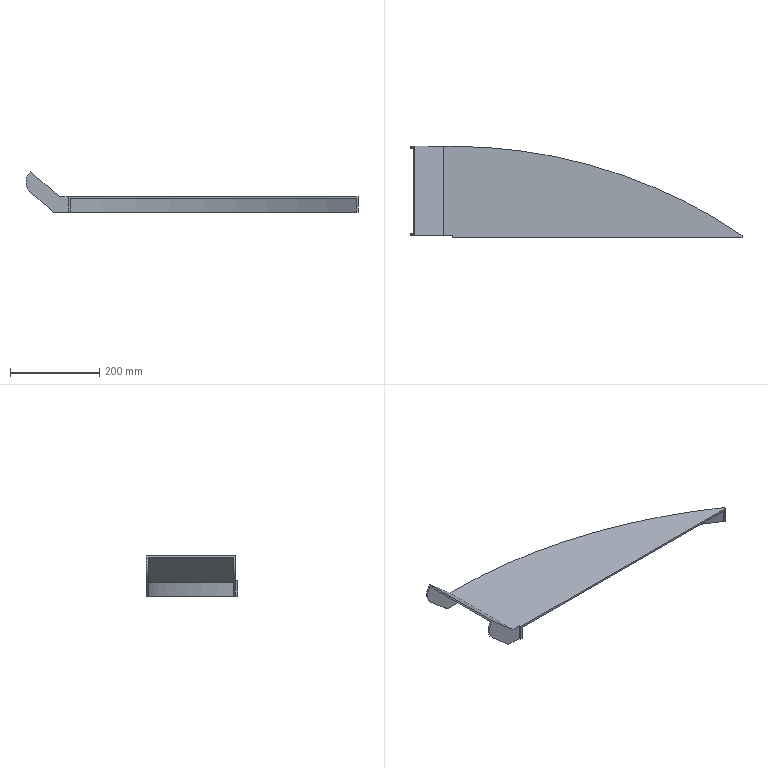Part | SolidWorks | features Shell 2, Extrusion 1, Fillet 1, ICE 1 | 1 solid | 22 faces | box 744.916 x 205 x 90.512 mm | volume 566343 mm3 | plane 18 | cylinder 4 | commonest cylinder face diameters 60 x2 2304 x1 2312 x1
STEP:
#1=CARTESIAN_POINT('',(-33.008,0.,0.));
#2=VERTEX_POINT('',#1);
#3=CARTESIAN_POINT('',(-33.008,4.,0.));
#4=VERTEX_POINT('',#3);
#5=CARTESIAN_POINT('',(-33.008,-125.702,0.));
#6=DIRECTION('',(0.,1.,0.));
#7=VECTOR('',#6,1000.);
#8=LINE('',#5,#7);
#9=EDGE_CURVE('',#2,#4,#8,.T.);
#10=ORIENTED_EDGE('',*,*,#9,.T.);
#11=CARTESIAN_POINT('',(4.,4.,0.));
#12=VERTEX_POINT('',#11);
#13=CARTESIAN_POINT('',(0.,4.,0.));
#14=DIRECTION('',(1.,0.,0.));
#15=VECTOR('',#14,1000.);
#16=LINE('',#13,#15);
#17=EDGE_CURVE('',#4,#12,#16,.T.);
#18=ORIENTED_EDGE('',*,*,#17,.T.);
#19=CARTESIAN_POINT('',(4.,-5.,0.));
#20=VERTEX_POINT('',#19);
#21=CARTESIAN_POINT('',(4.,-956.25,0.));
#22=DIRECTION('',(0.,-1.,0.));
#23=VECTOR('',#22,1000.);
#24=LINE('',#21,#23);
#25=EDGE_CURVE('',#12,#20,#24,.T.);
#26=ORIENTED_EDGE('',*,*,#25,.T.);
#27=CARTESIAN_POINT('',(0.,-5.,0.));
#28=VERTEX_POINT('',#27);
#29=CARTESIAN_POINT('',(0.,-5.,0.));
#30=DIRECTION('',(1.,0.,0.));
#31=VECTOR('',#30,1000.);
#32=LINE('',#29,#31);
#33=EDGE_CURVE('',#28,#20,#32,.T.);
#34=ORIENTED_EDGE('',*,*,#33,.F.);
#35=CARTESIAN_POINT('',(0.,0.,0.));
#36=VERTEX_POINT('',#35);
#37=CARTESIAN_POINT('',(0.,0.,0.));
#38=DIRECTION('',(0.,-1.,0.));
#39=VECTOR('',#38,1000.);
#40=LINE('',#37,#39);
#41=EDGE_CURVE('',#36,#28,#40,.T.);
#42=ORIENTED_EDGE('',*,*,#41,.F.);
#43=CARTESIAN_POINT('',(-20.,0.,0.));
#44=DIRECTION('',(1.,0.,0.));
#45=VECTOR('',#44,1000.);
#46=LINE('',#43,#45);
#47=EDGE_CURVE('',#2,#36,#46,.T.);
#48=ORIENTED_EDGE('',*,*,#47,.F.);
#49=EDGE_LOOP('',(#10,#18,#26,#34,#42,#48));
#50=FACE_OUTER_BOUND('',#49,.T.);
#51=CARTESIAN_POINT('',(0.,-956.25,0.));
#52=DIRECTION('',(0.,0.,-1.));
#53=DIRECTION('',(-1.,0.,0.));
#54=AXIS2_PLACEMENT_3D('',#51,#52,#53);
#55=PLANE('',#54);
#56=ADVANCED_FACE('',(#50),#55,.T.);
#57=CARTESIAN_POINT('',(0.,196.,0.));
#58=VERTEX_POINT('',#57);
#59=CARTESIAN_POINT('',(-33.008,196.,0.));
#60=VERTEX_POINT('',#59);
#61=CARTESIAN_POINT('',(0.,196.,0.));
#62=DIRECTION('',(-1.,0.,0.));
#63=VECTOR('',#62,1000.);
#64=LINE('',#61,#63);
#65=EDGE_CURVE('',#58,#60,#64,.T.);
#66=ORIENTED_EDGE('',*,*,#65,.T.);
#67=CARTESIAN_POINT('',(-33.008,200.,0.));
#68=VERTEX_POINT('',#67);
#69=CARTESIAN_POINT('',(-33.008,-125.702,0.));
#70=DIRECTION('',(0.,1.,0.));
#71=VECTOR('',#70,1000.);
#72=LINE('',#69,#71);
#73=EDGE_CURVE('',#60,#68,#72,.T.);
#74=ORIENTED_EDGE('',*,*,#73,.T.);
#75=CARTESIAN_POINT('',(0.,200.,0.));
#76=VERTEX_POINT('',#75);
#77=CARTESIAN_POINT('',(0.,200.,0.));
#78=DIRECTION('',(-1.,0.,0.));
#79=VECTOR('',#78,1000.);
#80=LINE('',#77,#79);
#81=EDGE_CURVE('',#76,#68,#80,.T.);
#82=ORIENTED_EDGE('',*,*,#81,.F.);
#83=CARTESIAN_POINT('',(650.,0.,0.));
#84=VERTEX_POINT('',#83);
#85=CARTESIAN_POINT('',(0.,-956.25,0.));
#86=DIRECTION('',(0.,0.,1.));
#87=DIRECTION('',(-1.,0.,0.));
#88=AXIS2_PLACEMENT_3D('',#85,#86,#87);
#89=CIRCLE('',#88,1156.25);
#90=EDGE_CURVE('',#84,#76,#89,.T.);
#91=ORIENTED_EDGE('',*,*,#90,.F.);
#92=CARTESIAN_POINT('',(650.,-5.,0.));
#93=VERTEX_POINT('',#92);
#94=CARTESIAN_POINT('',(650.,-5.,0.));
#95=DIRECTION('',(0.,1.,0.));
#96=VECTOR('',#95,1000.);
#97=LINE('',#94,#96);
#98=EDGE_CURVE('',#93,#84,#97,.T.);
#99=ORIENTED_EDGE('',*,*,#98,.F.);
#100=CARTESIAN_POINT('',(646.,-5.,0.));
#101=VERTEX_POINT('',#100);
#102=CARTESIAN_POINT('',(0.,-5.,0.));
#103=DIRECTION('',(1.,0.,0.));
#104=VECTOR('',#103,1000.);
#105=LINE('',#102,#104);
#106=EDGE_CURVE('',#101,#93,#105,.T.);
#107=ORIENTED_EDGE('',*,*,#106,.F.);
#108=CARTESIAN_POINT('',(646.,-2.12,0.));
#109=VERTEX_POINT('',#108);
#110=CARTESIAN_POINT('',(646.,-956.25,0.));
#111=DIRECTION('',(0.,1.,0.));
#112=VECTOR('',#111,1000.);
#113=LINE('',#110,#112);
#114=EDGE_CURVE('',#101,#109,#113,.T.);
#115=ORIENTED_EDGE('',*,*,#114,.T.);
#116=CARTESIAN_POINT('',(0.,-956.25,0.));
#117=DIRECTION('',(0.,0.,1.));
#118=DIRECTION('',(-1.,0.,0.));
#119=AXIS2_PLACEMENT_3D('',#116,#117,#118);
#120=CIRCLE('',#119,1152.25);
#121=EDGE_CURVE('',#109,#58,#120,.T.);
#122=ORIENTED_EDGE('',*,*,#121,.T.);
#123=EDGE_LOOP('',(#66,#74,#82,#91,#99,#107,#115,#122));
#124=FACE_OUTER_BOUND('',#123,.T.);
#125=CARTESIAN_POINT('',(0.,-956.25,0.));
#126=DIRECTION('',(0.,0.,-1.));
#127=DIRECTION('',(-1.,0.,0.));
#128=AXIS2_PLACEMENT_3D('',#125,#126,#127);
#129=PLANE('',#128);
#130=ADVANCED_FACE('',(#124),#129,.T.);
#131=CARTESIAN_POINT('',(-84.369,200.,90.512));
#132=VERTEX_POINT('',#131);
#133=CARTESIAN_POINT('',(-87.634,200.,86.726));
#134=VERTEX_POINT('',#133);
#135=CARTESIAN_POINT('',(-93.149,200.,80.332));
#136=DIRECTION('',(-0.6531,0.,-0.7573));
#137=VECTOR('',#136,1000.);
#138=LINE('',#135,#137);
#139=EDGE_CURVE('',#132,#134,#138,.T.);
#140=ORIENTED_EDGE('',*,*,#139,.T.);
#141=CARTESIAN_POINT('',(-87.634,196.,86.726));
#142=VERTEX_POINT('',#141);
#143=CARTESIAN_POINT('',(-87.634,-125.702,86.726));
#144=DIRECTION('',(0.,-1.,0.));
#145=VECTOR('',#144,1000.);
#146=LINE('',#143,#145);
#147=EDGE_CURVE('',#134,#142,#146,.T.);
#148=ORIENTED_EDGE('',*,*,#147,.T.);
#149=CARTESIAN_POINT('',(-86.981,196.,87.483));
#150=VERTEX_POINT('',#149);
#151=CARTESIAN_POINT('',(-93.149,196.,80.332));
#152=DIRECTION('',(-0.6531,0.,-0.7573));
#153=VECTOR('',#152,1000.);
#154=LINE('',#151,#153);
#155=EDGE_CURVE('',#150,#142,#154,.T.);
#156=ORIENTED_EDGE('',*,*,#155,.F.);
#157=CARTESIAN_POINT('',(-86.981,4.,87.483));
#158=VERTEX_POINT('',#157);
#159=CARTESIAN_POINT('',(-86.981,-125.702,87.483));
#160=DIRECTION('',(0.,1.,0.));
#161=VECTOR('',#160,1000.);
#162=LINE('',#159,#161);
#163=EDGE_CURVE('',#158,#150,#162,.T.);
#164=ORIENTED_EDGE('',*,*,#163,.F.);
#165=CARTESIAN_POINT('',(-87.634,4.,86.726));
#166=VERTEX_POINT('',#165);
#167=CARTESIAN_POINT('',(-93.149,4.,80.332));
#168=DIRECTION('',(0.6531,0.,0.7573));
#169=VECTOR('',#168,1000.);
#170=LINE('',#167,#169);
#171=EDGE_CURVE('',#166,#158,#170,.T.);
#172=ORIENTED_EDGE('',*,*,#171,.F.);
#173=CARTESIAN_POINT('',(-87.634,0.,86.726));
#174=VERTEX_POINT('',#173);
#175=CARTESIAN_POINT('',(-87.634,-125.702,86.726));
#176=DIRECTION('',(0.,-1.,0.));
#177=VECTOR('',#176,1000.);
#178=LINE('',#175,#177);
#179=EDGE_CURVE('',#166,#174,#178,.T.);
#180=ORIENTED_EDGE('',*,*,#179,.T.);
#181=CARTESIAN_POINT('',(-84.369,0.,90.512));
#182=VERTEX_POINT('',#181);
#183=CARTESIAN_POINT('',(-93.149,0.,80.332));
#184=DIRECTION('',(0.6531,0.,0.7573));
#185=VECTOR('',#184,1000.);
#186=LINE('',#183,#185);
#187=EDGE_CURVE('',#174,#182,#186,.T.);
#188=ORIENTED_EDGE('',*,*,#187,.T.);
#189=CARTESIAN_POINT('',(-84.369,-125.702,90.512));
#190=DIRECTION('',(0.,1.,0.));
#191=VECTOR('',#190,1000.);
#192=LINE('',#189,#191);
#193=EDGE_CURVE('',#182,#132,#192,.T.);
#194=ORIENTED_EDGE('',*,*,#193,.T.);
#195=EDGE_LOOP('',(#140,#148,#156,#164,#172,#180,#188,#194));
#196=FACE_OUTER_BOUND('',#195,.T.);
#197=CARTESIAN_POINT('',(-93.149,-125.702,80.332));
#198=DIRECTION('',(0.7573,0.,-0.6531));
#199=DIRECTION('',(-0.6531,0.,-0.7573));
#200=AXIS2_PLACEMENT_3D('',#197,#198,#199);
#201=PLANE('',#200);
#202=ADVANCED_FACE('',(#196),#201,.F.);
#203=CARTESIAN_POINT('',(-84.509,0.,44.415));
#204=VERTEX_POINT('',#203);
#205=CARTESIAN_POINT('',(-14.079,0.,-16.325));
#206=DIRECTION('',(-0.7573,0.,0.6531));
#207=VECTOR('',#206,1000.);
#208=LINE('',#205,#207);
#209=EDGE_CURVE('',#2,#204,#208,.T.);
#210=ORIENTED_EDGE('',*,*,#209,.T.);
#211=CARTESIAN_POINT('',(-84.509,4.,44.415));
#212=VERTEX_POINT('',#211);
#213=CARTESIAN_POINT('',(-84.509,-125.702,44.415));
#214=DIRECTION('',(0.,1.,0.));
#215=VECTOR('',#214,1000.);
#216=LINE('',#213,#215);
#217=EDGE_CURVE('',#204,#212,#216,.T.);
#218=ORIENTED_EDGE('',*,*,#217,.T.);
#219=CARTESIAN_POINT('',(-14.079,4.,-16.325));
#220=DIRECTION('',(-0.7573,0.,0.6531));
#221=VECTOR('',#220,1000.);
#222=LINE('',#219,#221);
#223=EDGE_CURVE('',#4,#212,#222,.T.);
#224=ORIENTED_EDGE('',*,*,#223,.F.);
#225=ORIENTED_EDGE('',*,*,#9,.F.);
#226=EDGE_LOOP('',(#210,#218,#224,#225));
#227=FACE_OUTER_BOUND('',#226,.T.);
#228=CARTESIAN_POINT('',(-14.079,-125.702,-16.325));
#229=DIRECTION('',(0.6531,0.,0.7573));
#230=DIRECTION('',(0.7573,0.,-0.6531));
#231=AXIS2_PLACEMENT_3D('',#228,#229,#230);
#232=PLANE('',#231);
#233=ADVANCED_FACE('',(#227),#232,.F.);
#234=CARTESIAN_POINT('',(-84.509,196.,44.415));
#235=VERTEX_POINT('',#234);
#236=CARTESIAN_POINT('',(-14.079,196.,-16.325));
#237=DIRECTION('',(0.7573,0.,-0.6531));
#238=VECTOR('',#237,1000.);
#239=LINE('',#236,#238);
#240=EDGE_CURVE('',#235,#60,#239,.T.);
#241=ORIENTED_EDGE('',*,*,#240,.F.);
#242=CARTESIAN_POINT('',(-84.509,200.,44.415));
#243=VERTEX_POINT('',#242);
#244=CARTESIAN_POINT('',(-84.509,-125.702,44.415));
#245=DIRECTION('',(0.,1.,0.));
#246=VECTOR('',#245,1000.);
#247=LINE('',#244,#246);
#248=EDGE_CURVE('',#235,#243,#247,.T.);
#249=ORIENTED_EDGE('',*,*,#248,.T.);
#250=CARTESIAN_POINT('',(-14.079,200.,-16.325));
#251=DIRECTION('',(0.7573,0.,-0.6531));
#252=VECTOR('',#251,1000.);
#253=LINE('',#250,#252);
#254=EDGE_CURVE('',#243,#68,#253,.T.);
#255=ORIENTED_EDGE('',*,*,#254,.T.);
#256=ORIENTED_EDGE('',*,*,#73,.F.);
#257=EDGE_LOOP('',(#241,#249,#255,#256));
#258=FACE_OUTER_BOUND('',#257,.T.);
#259=CARTESIAN_POINT('',(-14.079,-125.702,-16.325));
#260=DIRECTION('',(0.6531,0.,0.7573));
#261=DIRECTION('',(0.7573,0.,-0.6531));
#262=AXIS2_PLACEMENT_3D('',#259,#260,#261);
#263=PLANE('',#262);
#264=ADVANCED_FACE('',(#258),#263,.F.);
#265=ORIENTED_EDGE('',*,*,#187,.F.);
#266=CARTESIAN_POINT('',(-64.916,0.,67.133));
#267=DIRECTION('',(0.,-1.,0.));
#268=DIRECTION('',(0.,0.,1.));
#269=AXIS2_PLACEMENT_3D('',#266,#267,#268);
#270=CIRCLE('',#269,30.);
#271=EDGE_CURVE('',#174,#204,#270,.T.);
#272=ORIENTED_EDGE('',*,*,#271,.T.);
#273=ORIENTED_EDGE('',*,*,#209,.F.);
#274=ORIENTED_EDGE('',*,*,#47,.T.);
#275=CARTESIAN_POINT('',(0.,0.,35.));
#276=VERTEX_POINT('',#275);
#277=CARTESIAN_POINT('',(0.,0.,35.));
#278=DIRECTION('',(0.,0.,-1.));
#279=VECTOR('',#278,1000.);
#280=LINE('',#277,#279);
#281=EDGE_CURVE('',#276,#36,#280,.T.);
#282=ORIENTED_EDGE('',*,*,#281,.F.);
#283=CARTESIAN_POINT('',(-20.,0.,35.));
#284=VERTEX_POINT('',#283);
#285=CARTESIAN_POINT('',(-20.,0.,35.));
#286=DIRECTION('',(1.,0.,0.));
#287=VECTOR('',#286,1000.);
#288=LINE('',#285,#287);
#289=EDGE_CURVE('',#284,#276,#288,.T.);
#290=ORIENTED_EDGE('',*,*,#289,.F.);
#291=CARTESIAN_POINT('',(8.78,0.,10.18));
#292=DIRECTION('',(0.7573,0.,-0.6531));
#293=VECTOR('',#292,1000.);
#294=LINE('',#291,#293);
#295=EDGE_CURVE('',#182,#284,#294,.T.);
#296=ORIENTED_EDGE('',*,*,#295,.F.);
#297=EDGE_LOOP('',(#265,#272,#273,#274,#282,#290,#296));
#298=FACE_OUTER_BOUND('',#297,.T.);
#299=CARTESIAN_POINT('',(-20.,0.,35.));
#300=DIRECTION('',(0.,1.,0.));
#301=DIRECTION('',(0.,0.,1.));
#302=AXIS2_PLACEMENT_3D('',#299,#300,#301);
#303=PLANE('',#302);
#304=ADVANCED_FACE('',(#298),#303,.F.);
#305=ORIENTED_EDGE('',*,*,#41,.T.);
#306=CARTESIAN_POINT('',(0.,-5.,35.));
#307=VERTEX_POINT('',#306);
#308=CARTESIAN_POINT('',(0.,-5.,35.));
#309=DIRECTION('',(0.,0.,-1.));
#310=VECTOR('',#309,1000.);
#311=LINE('',#308,#310);
#312=EDGE_CURVE('',#307,#28,#311,.T.);
#313=ORIENTED_EDGE('',*,*,#312,.F.);
#314=CARTESIAN_POINT('',(0.,0.,35.));
#315=DIRECTION('',(0.,-1.,0.));
#316=VECTOR('',#315,1000.);
#317=LINE('',#314,#316);
#318=EDGE_CURVE('',#276,#307,#317,.T.);
#319=ORIENTED_EDGE('',*,*,#318,.F.);
#320=ORIENTED_EDGE('',*,*,#281,.T.);
#321=EDGE_LOOP('',(#305,#313,#319,#320));
#322=FACE_OUTER_BOUND('',#321,.T.);
#323=CARTESIAN_POINT('',(0.,0.,35.));
#324=DIRECTION('',(1.,0.,0.));
#325=DIRECTION('',(0.,1.,0.));
#326=AXIS2_PLACEMENT_3D('',#323,#324,#325);
#327=PLANE('',#326);
#328=ADVANCED_FACE('',(#322),#327,.F.);
#329=CARTESIAN_POINT('',(4.,-5.,31.));
#330=VERTEX_POINT('',#329);
#331=CARTESIAN_POINT('',(646.,-5.,31.));
#332=VERTEX_POINT('',#331);
#333=CARTESIAN_POINT('',(0.,-5.,31.));
#334=DIRECTION('',(1.,0.,0.));
#335=VECTOR('',#334,1000.);
#336=LINE('',#333,#335);
#337=EDGE_CURVE('',#330,#332,#336,.T.);
#338=ORIENTED_EDGE('',*,*,#337,.T.);
#339=CARTESIAN_POINT('',(646.,-5.,35.));
#340=DIRECTION('',(0.,0.,-1.));
#341=VECTOR('',#340,1000.);
#342=LINE('',#339,#341);
#343=EDGE_CURVE('',#332,#101,#342,.T.);
#344=ORIENTED_EDGE('',*,*,#343,.T.);
#345=ORIENTED_EDGE('',*,*,#106,.T.);
#346=CARTESIAN_POINT('',(650.,-5.,35.));
#347=VERTEX_POINT('',#346);
#348=CARTESIAN_POINT('',(650.,-5.,35.));
#349=DIRECTION('',(0.,0.,-1.));
#350=VECTOR('',#349,1000.);
#351=LINE('',#348,#350);
#352=EDGE_CURVE('',#347,#93,#351,.T.);
#353=ORIENTED_EDGE('',*,*,#352,.F.);
#354=CARTESIAN_POINT('',(0.,-5.,35.));
#355=DIRECTION('',(1.,0.,0.));
#356=VECTOR('',#355,1000.);
#357=LINE('',#354,#356);
#358=EDGE_CURVE('',#307,#347,#357,.T.);
#359=ORIENTED_EDGE('',*,*,#358,.F.);
#360=ORIENTED_EDGE('',*,*,#312,.T.);
#361=ORIENTED_EDGE('',*,*,#33,.T.);
#362=CARTESIAN_POINT('',(4.,-5.,35.));
#363=DIRECTION('',(0.,0.,-1.));
#364=VECTOR('',#363,1000.);
#365=LINE('',#362,#364);
#366=EDGE_CURVE('',#330,#20,#365,.T.);
#367=ORIENTED_EDGE('',*,*,#366,.F.);
#368=EDGE_LOOP('',(#338,#344,#345,#353,#359,#360,#361,#367));
#369=FACE_OUTER_BOUND('',#368,.T.);
#370=CARTESIAN_POINT('',(0.,-5.,35.));
#371=DIRECTION('',(0.,1.,0.));
#372=DIRECTION('',(0.,0.,1.));
#373=AXIS2_PLACEMENT_3D('',#370,#371,#372);
#374=PLANE('',#373);
#375=ADVANCED_FACE('',(#369),#374,.F.);
#376=ORIENTED_EDGE('',*,*,#98,.T.);
#377=CARTESIAN_POINT('',(650.,0.,35.));
#378=VERTEX_POINT('',#377);
#379=CARTESIAN_POINT('',(650.,0.,35.));
#380=DIRECTION('',(0.,0.,-1.));
#381=VECTOR('',#380,1000.);
#382=LINE('',#379,#381);
#383=EDGE_CURVE('',#378,#84,#382,.T.);
#384=ORIENTED_EDGE('',*,*,#383,.F.);
#385=CARTESIAN_POINT('',(650.,-5.,35.));
#386=DIRECTION('',(0.,1.,0.));
#387=VECTOR('',#386,1000.);
#388=LINE('',#385,#387);
#389=EDGE_CURVE('',#347,#378,#388,.T.);
#390=ORIENTED_EDGE('',*,*,#389,.F.);
#391=ORIENTED_EDGE('',*,*,#352,.T.);
#392=EDGE_LOOP('',(#376,#384,#390,#391));
#393=FACE_OUTER_BOUND('',#392,.T.);
#394=CARTESIAN_POINT('',(650.,-5.,35.));
#395=DIRECTION('',(-1.,0.,0.));
#396=DIRECTION('',(0.,0.,1.));
#397=AXIS2_PLACEMENT_3D('',#394,#395,#396);
#398=PLANE('',#397);
#399=ADVANCED_FACE('',(#393),#398,.F.);
#400=ORIENTED_EDGE('',*,*,#90,.T.);
#401=CARTESIAN_POINT('',(0.,200.,35.));
#402=VERTEX_POINT('',#401);
#403=CARTESIAN_POINT('',(0.,200.,35.));
#404=DIRECTION('',(0.,0.,-1.));
#405=VECTOR('',#404,1000.);
#406=LINE('',#403,#405);
#407=EDGE_CURVE('',#402,#76,#406,.T.);
#408=ORIENTED_EDGE('',*,*,#407,.F.);
#409=CARTESIAN_POINT('',(0.,-956.25,35.));
#410=DIRECTION('',(0.,0.,1.));
#411=DIRECTION('',(-1.,0.,0.));
#412=AXIS2_PLACEMENT_3D('',#409,#410,#411);
#413=CIRCLE('',#412,1156.25);
#414=EDGE_CURVE('',#378,#402,#413,.T.);
#415=ORIENTED_EDGE('',*,*,#414,.F.);
#416=ORIENTED_EDGE('',*,*,#383,.T.);
#417=EDGE_LOOP('',(#400,#408,#415,#416));
#418=FACE_OUTER_BOUND('',#417,.T.);
#419=CARTESIAN_POINT('',(0.,-956.25,35.));
#420=DIRECTION('',(0.,0.,-1.));
#421=DIRECTION('',(-1.,0.,0.));
#422=AXIS2_PLACEMENT_3D('',#419,#420,#421);
#423=CYLINDRICAL_SURFACE('',#422,1156.25);
#424=ADVANCED_FACE('',(#418),#423,.T.);
#425=ORIENTED_EDGE('',*,*,#254,.F.);
#426=CARTESIAN_POINT('',(-64.916,200.,67.133));
#427=DIRECTION('',(0.,1.,0.));
#428=DIRECTION('',(0.,0.,-1.));
#429=AXIS2_PLACEMENT_3D('',#426,#427,#428);
#430=CIRCLE('',#429,30.);
#431=EDGE_CURVE('',#243,#134,#430,.T.);
#432=ORIENTED_EDGE('',*,*,#431,.T.);
#433=ORIENTED_EDGE('',*,*,#139,.F.);
#434=CARTESIAN_POINT('',(-20.,200.,35.));
#435=VERTEX_POINT('',#434);
#436=CARTESIAN_POINT('',(8.78,200.,10.18));
#437=DIRECTION('',(-0.7573,0.,0.6531));
#438=VECTOR('',#437,1000.);
#439=LINE('',#436,#438);
#440=EDGE_CURVE('',#435,#132,#439,.T.);
#441=ORIENTED_EDGE('',*,*,#440,.F.);
#442=CARTESIAN_POINT('',(0.,200.,35.));
#443=DIRECTION('',(-1.,0.,0.));
#444=VECTOR('',#443,1000.);
#445=LINE('',#442,#444);
#446=EDGE_CURVE('',#402,#435,#445,.T.);
#447=ORIENTED_EDGE('',*,*,#446,.F.);
#448=ORIENTED_EDGE('',*,*,#407,.T.);
#449=ORIENTED_EDGE('',*,*,#81,.T.);
#450=EDGE_LOOP('',(#425,#432,#433,#441,#447,#448,#449));
#451=FACE_OUTER_BOUND('',#450,.T.);
#452=CARTESIAN_POINT('',(0.,200.,35.));
#453=DIRECTION('',(0.,-1.,0.));
#454=DIRECTION('',(0.,0.,-1.));
#455=AXIS2_PLACEMENT_3D('',#452,#453,#454);
#456=PLANE('',#455);
#457=ADVANCED_FACE('',(#451),#456,.F.);
#458=ORIENTED_EDGE('',*,*,#289,.T.);
#459=ORIENTED_EDGE('',*,*,#318,.T.);
#460=ORIENTED_EDGE('',*,*,#358,.T.);
#461=ORIENTED_EDGE('',*,*,#389,.T.);
#462=ORIENTED_EDGE('',*,*,#414,.T.);
#463=ORIENTED_EDGE('',*,*,#446,.T.);
#464=CARTESIAN_POINT('',(-20.,200.,35.));
#465=DIRECTION('',(0.,-1.,0.));
#466=VECTOR('',#465,1000.);
#467=LINE('',#464,#466);
#468=EDGE_CURVE('',#435,#284,#467,.T.);
#469=ORIENTED_EDGE('',*,*,#468,.T.);
#470=EDGE_LOOP('',(#458,#459,#460,#461,#462,#463,#469));
#471=FACE_OUTER_BOUND('',#470,.T.);
#472=CARTESIAN_POINT('',(0.,-956.25,35.));
#473=DIRECTION('',(0.,0.,-1.));
#474=DIRECTION('',(-1.,0.,0.));
#475=AXIS2_PLACEMENT_3D('',#472,#473,#474);
#476=PLANE('',#475);
#477=ADVANCED_FACE('',(#471),#476,.F.);
#478=ORIENTED_EDGE('',*,*,#223,.T.);
#479=CARTESIAN_POINT('',(-64.916,4.,67.133));
#480=DIRECTION('',(0.,1.,0.));
#481=DIRECTION('',(0.,0.,1.));
#482=AXIS2_PLACEMENT_3D('',#479,#480,#481);
#483=CIRCLE('',#482,30.);
#484=EDGE_CURVE('',#212,#166,#483,.T.);
#485=ORIENTED_EDGE('',*,*,#484,.T.);
#486=ORIENTED_EDGE('',*,*,#171,.T.);
#487=CARTESIAN_POINT('',(-21.487,4.,31.));
#488=VERTEX_POINT('',#487);
#489=CARTESIAN_POINT('',(6.167,4.,7.151));
#490=DIRECTION('',(0.7573,0.,-0.6531));
#491=VECTOR('',#490,1000.);
#492=LINE('',#489,#491);
#493=EDGE_CURVE('',#158,#488,#492,.T.);
#494=ORIENTED_EDGE('',*,*,#493,.T.);
#495=CARTESIAN_POINT('',(4.,4.,31.));
#496=VERTEX_POINT('',#495);
#497=CARTESIAN_POINT('',(0.,4.,31.));
#498=DIRECTION('',(1.,0.,0.));
#499=VECTOR('',#498,1000.);
#500=LINE('',#497,#499);
#501=EDGE_CURVE('',#488,#496,#500,.T.);
#502=ORIENTED_EDGE('',*,*,#501,.T.);
#503=CARTESIAN_POINT('',(4.,4.,35.));
#504=DIRECTION('',(0.,0.,-1.));
#505=VECTOR('',#504,1000.);
#506=LINE('',#503,#505);
#507=EDGE_CURVE('',#496,#12,#506,.T.);
#508=ORIENTED_EDGE('',*,*,#507,.T.);
#509=ORIENTED_EDGE('',*,*,#17,.F.);
#510=EDGE_LOOP('',(#478,#485,#486,#494,#502,#508,#509));
#511=FACE_OUTER_BOUND('',#510,.T.);
#512=CARTESIAN_POINT('',(-20.,4.,35.));
#513=DIRECTION('',(0.,1.,0.));
#514=DIRECTION('',(0.,0.,1.));
#515=AXIS2_PLACEMENT_3D('',#512,#513,#514);
#516=PLANE('',#515);
#517=ADVANCED_FACE('',(#511),#516,.T.);
#518=ORIENTED_EDGE('',*,*,#25,.F.);
#519=ORIENTED_EDGE('',*,*,#507,.F.);
#520=CARTESIAN_POINT('',(4.,-956.25,31.));
#521=DIRECTION('',(0.,-1.,0.));
#522=VECTOR('',#521,1000.);
#523=LINE('',#520,#522);
#524=EDGE_CURVE('',#496,#330,#523,.T.);
#525=ORIENTED_EDGE('',*,*,#524,.T.);
#526=ORIENTED_EDGE('',*,*,#366,.T.);
#527=EDGE_LOOP('',(#518,#519,#525,#526));
#528=FACE_OUTER_BOUND('',#527,.T.);
#529=CARTESIAN_POINT('',(4.,0.,35.));
#530=DIRECTION('',(1.,0.,0.));
#531=DIRECTION('',(0.,1.,0.));
#532=AXIS2_PLACEMENT_3D('',#529,#530,#531);
#533=PLANE('',#532);
#534=ADVANCED_FACE('',(#528),#533,.T.);
#535=ORIENTED_EDGE('',*,*,#114,.F.);
#536=ORIENTED_EDGE('',*,*,#343,.F.);
#537=CARTESIAN_POINT('',(646.,-2.12,31.));
#538=VERTEX_POINT('',#537);
#539=CARTESIAN_POINT('',(646.,-956.25,31.));
#540=DIRECTION('',(0.,1.,0.));
#541=VECTOR('',#540,1000.);
#542=LINE('',#539,#541);
#543=EDGE_CURVE('',#332,#538,#542,.T.);
#544=ORIENTED_EDGE('',*,*,#543,.T.);
#545=CARTESIAN_POINT('',(646.,-2.12,31.));
#546=DIRECTION('',(0.,0.,-1.));
#547=VECTOR('',#546,1000.);
#548=LINE('',#545,#547);
#549=EDGE_CURVE('',#538,#109,#548,.T.);
#550=ORIENTED_EDGE('',*,*,#549,.T.);
#551=EDGE_LOOP('',(#535,#536,#544,#550));
#552=FACE_OUTER_BOUND('',#551,.T.);
#553=CARTESIAN_POINT('',(646.,-5.,35.));
#554=DIRECTION('',(-1.,0.,0.));
#555=DIRECTION('',(0.,0.,1.));
#556=AXIS2_PLACEMENT_3D('',#553,#554,#555);
#557=PLANE('',#556);
#558=ADVANCED_FACE('',(#552),#557,.T.);
#559=ORIENTED_EDGE('',*,*,#121,.F.);
#560=ORIENTED_EDGE('',*,*,#549,.F.);
#561=CARTESIAN_POINT('',(0.,196.,31.));
#562=VERTEX_POINT('',#561);
#563=CARTESIAN_POINT('',(0.,-956.25,31.));
#564=DIRECTION('',(0.,0.,1.));
#565=DIRECTION('',(-1.,0.,0.));
#566=AXIS2_PLACEMENT_3D('',#563,#564,#565);
#567=CIRCLE('',#566,1152.25);
#568=EDGE_CURVE('',#538,#562,#567,.T.);
#569=ORIENTED_EDGE('',*,*,#568,.T.);
#570=CARTESIAN_POINT('',(0.,196.,35.));
#571=DIRECTION('',(0.,0.,-1.));
#572=VECTOR('',#571,1000.);
#573=LINE('',#570,#572);
#574=EDGE_CURVE('',#562,#58,#573,.T.);
#575=ORIENTED_EDGE('',*,*,#574,.T.);
#576=EDGE_LOOP('',(#559,#560,#569,#575));
#577=FACE_OUTER_BOUND('',#576,.T.);
#578=CARTESIAN_POINT('',(0.,-956.25,35.));
#579=DIRECTION('',(0.,0.,-1.));
#580=DIRECTION('',(-1.,0.,0.));
#581=AXIS2_PLACEMENT_3D('',#578,#579,#580);
#582=CYLINDRICAL_SURFACE('',#581,1152.25);
#583=ADVANCED_FACE('',(#577),#582,.F.);
#584=ORIENTED_EDGE('',*,*,#155,.T.);
#585=CARTESIAN_POINT('',(-64.916,196.,67.133));
#586=DIRECTION('',(0.,-1.,0.));
#587=DIRECTION('',(0.,0.,-1.));
#588=AXIS2_PLACEMENT_3D('',#585,#586,#587);
#589=CIRCLE('',#588,30.);
#590=EDGE_CURVE('',#142,#235,#589,.T.);
#591=ORIENTED_EDGE('',*,*,#590,.T.);
#592=ORIENTED_EDGE('',*,*,#240,.T.);
#593=ORIENTED_EDGE('',*,*,#65,.F.);
#594=ORIENTED_EDGE('',*,*,#574,.F.);
#595=CARTESIAN_POINT('',(-21.487,196.,31.));
#596=VERTEX_POINT('',#595);
#597=CARTESIAN_POINT('',(0.,196.,31.));
#598=DIRECTION('',(-1.,0.,0.));
#599=VECTOR('',#598,1000.);
#600=LINE('',#597,#599);
#601=EDGE_CURVE('',#562,#596,#600,.T.);
#602=ORIENTED_EDGE('',*,*,#601,.T.);
#603=CARTESIAN_POINT('',(6.167,196.,7.151));
#604=DIRECTION('',(-0.7573,0.,0.6531));
#605=VECTOR('',#604,1000.);
#606=LINE('',#603,#605);
#607=EDGE_CURVE('',#596,#150,#606,.T.);
#608=ORIENTED_EDGE('',*,*,#607,.T.);
#609=EDGE_LOOP('',(#584,#591,#592,#593,#594,#602,#608));
#610=FACE_OUTER_BOUND('',#609,.T.);
#611=CARTESIAN_POINT('',(0.,196.,35.));
#612=DIRECTION('',(0.,-1.,0.));
#613=DIRECTION('',(0.,0.,-1.));
#614=AXIS2_PLACEMENT_3D('',#611,#612,#613);
#615=PLANE('',#614);
#616=ADVANCED_FACE('',(#610),#615,.T.);
#617=ORIENTED_EDGE('',*,*,#501,.F.);
#618=CARTESIAN_POINT('',(-21.487,-125.702,31.));
#619=DIRECTION('',(0.,-1.,0.));
#620=VECTOR('',#619,1000.);
#621=LINE('',#618,#620);
#622=EDGE_CURVE('',#596,#488,#621,.T.);
#623=ORIENTED_EDGE('',*,*,#622,.F.);
#624=ORIENTED_EDGE('',*,*,#601,.F.);
#625=ORIENTED_EDGE('',*,*,#568,.F.);
#626=ORIENTED_EDGE('',*,*,#543,.F.);
#627=ORIENTED_EDGE('',*,*,#337,.F.);
#628=ORIENTED_EDGE('',*,*,#524,.F.);
#629=EDGE_LOOP('',(#617,#623,#624,#625,#626,#627,#628));
#630=FACE_OUTER_BOUND('',#629,.T.);
#631=CARTESIAN_POINT('',(0.,-956.25,31.));
#632=DIRECTION('',(0.,0.,-1.));
#633=DIRECTION('',(-1.,0.,0.));
#634=AXIS2_PLACEMENT_3D('',#631,#632,#633);
#635=PLANE('',#634);
#636=ADVANCED_FACE('',(#630),#635,.T.);
#637=ORIENTED_EDGE('',*,*,#193,.F.);
#638=ORIENTED_EDGE('',*,*,#295,.T.);
#639=ORIENTED_EDGE('',*,*,#468,.F.);
#640=ORIENTED_EDGE('',*,*,#440,.T.);
#641=EDGE_LOOP('',(#637,#638,#639,#640));
#642=FACE_OUTER_BOUND('',#641,.T.);
#643=CARTESIAN_POINT('',(8.78,-125.702,10.18));
#644=DIRECTION('',(-0.6531,0.,-0.7573));
#645=DIRECTION('',(-0.7573,0.,0.6531));
#646=AXIS2_PLACEMENT_3D('',#643,#644,#645);
#647=PLANE('',#646);
#648=ADVANCED_FACE('',(#642),#647,.F.);
#649=ORIENTED_EDGE('',*,*,#163,.T.);
#650=ORIENTED_EDGE('',*,*,#607,.F.);
#651=ORIENTED_EDGE('',*,*,#622,.T.);
#652=ORIENTED_EDGE('',*,*,#493,.F.);
#653=EDGE_LOOP('',(#649,#650,#651,#652));
#654=FACE_OUTER_BOUND('',#653,.T.);
#655=CARTESIAN_POINT('',(6.167,-125.702,7.151));
#656=DIRECTION('',(-0.6531,0.,-0.7573));
#657=DIRECTION('',(-0.7573,0.,0.6531));
#658=AXIS2_PLACEMENT_3D('',#655,#656,#657);
#659=PLANE('',#658);
#660=ADVANCED_FACE('',(#654),#659,.T.);
#661=ORIENTED_EDGE('',*,*,#590,.F.);
#662=ORIENTED_EDGE('',*,*,#147,.F.);
#663=ORIENTED_EDGE('',*,*,#431,.F.);
#664=ORIENTED_EDGE('',*,*,#248,.F.);
#665=EDGE_LOOP('',(#661,#662,#663,#664));
#666=FACE_OUTER_BOUND('',#665,.T.);
#667=CARTESIAN_POINT('',(-64.916,-125.702,67.133));
#668=DIRECTION('',(0.,1.,0.));
#669=DIRECTION('',(0.,0.,1.));
#670=AXIS2_PLACEMENT_3D('',#667,#668,#669);
#671=CYLINDRICAL_SURFACE('',#670,30.);
#672=ADVANCED_FACE('',(#666),#671,.T.);
#673=ORIENTED_EDGE('',*,*,#271,.F.);
#674=ORIENTED_EDGE('',*,*,#179,.F.);
#675=ORIENTED_EDGE('',*,*,#484,.F.);
#676=ORIENTED_EDGE('',*,*,#217,.F.);
#677=EDGE_LOOP('',(#673,#674,#675,#676));
#678=FACE_OUTER_BOUND('',#677,.T.);
#679=CARTESIAN_POINT('',(-64.916,-125.702,67.133));
#680=DIRECTION('',(0.,1.,0.));
#681=DIRECTION('',(0.,0.,1.));
#682=AXIS2_PLACEMENT_3D('',#679,#680,#681);
#683=CYLINDRICAL_SURFACE('',#682,30.);
#684=ADVANCED_FACE('',(#678),#683,.T.);
#685=CLOSED_SHELL('',(#56,#130,#202,#233,#264,#304,#328,#375,#399,#424,#457,#477,#517,#534,#558,#583,#616,#636,#648,#660,#672,#684));
#686=MANIFOLD_SOLID_BREP('',#685);
#687=CARTESIAN_POINT('',(0.,0.,0.));
#688=DIRECTION('',(0.,0.,1.));
#689=DIRECTION('',(1.,0.,0.));
#690=AXIS2_PLACEMENT_3D('',#687,#688,#689);
#691=(LENGTH_UNIT()NAMED_UNIT(*)SI_UNIT(.MILLI.,.METRE.));
#692=UNCERTAINTY_MEASURE_WITH_UNIT(LENGTH_MEASURE(0.00001),#691,'','');
#693=(NAMED_UNIT(*)PLANE_ANGLE_UNIT()SI_UNIT($,.RADIAN.));
#694=(NAMED_UNIT(*)SI_UNIT($,.STERADIAN.)SOLID_ANGLE_UNIT());
#695=(GEOMETRIC_REPRESENTATION_CONTEXT(3)GLOBAL_UNCERTAINTY_ASSIGNED_CONTEXT((#692))GLOBAL_UNIT_ASSIGNED_CONTEXT((#691,#693,#694))REPRESENTATION_CONTEXT('',''));
#696=ADVANCED_BREP_SHAPE_REPRESENTATION('',(#686,#690),#695);